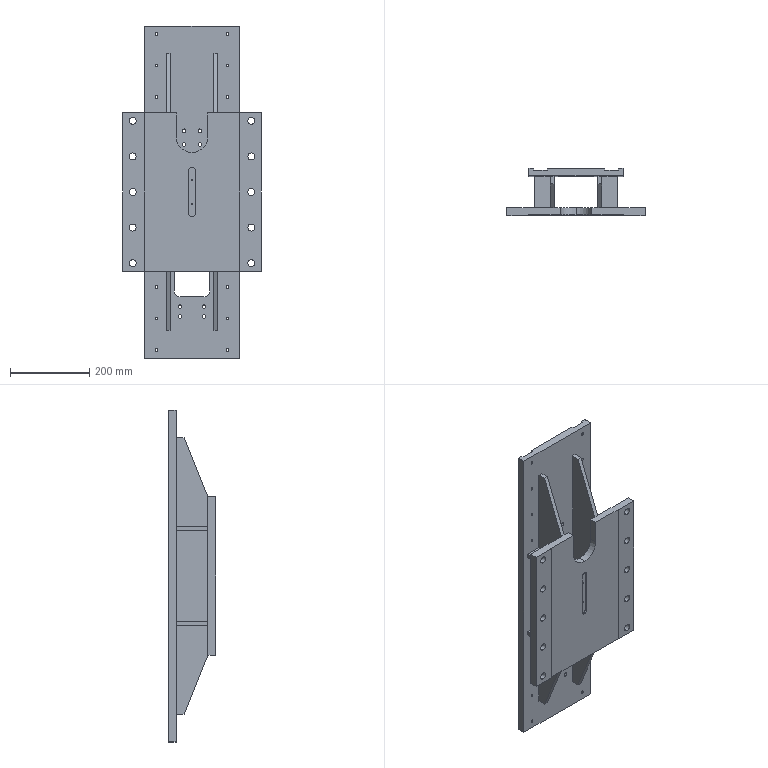Part | STEP file | YCD14007A-08.02.04-Lift Connecting Plate-A2 | 1 solid | 209 faces | box 350 x 120 x 840 mm | volume 6654945 mm3 | cylinder 121 | plane 76 | cone 12 | commonest cylinder face diameters 6.8 x44 17.5 x20 9 x16 15 x16 5 x12 4.2 x4